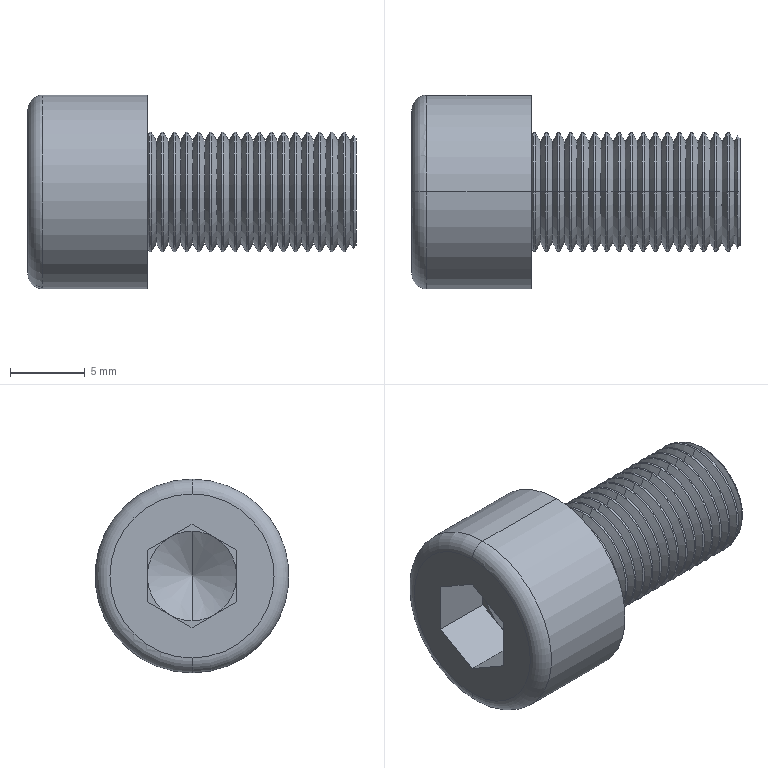Part | STEP file | PN_0011_Default<As Machined> | 1 solid | 148 faces | box 22 x 13 x 13 mm | volume 1485 mm3 | cone 84 | cylinder 42 | plane 20 | torus 2 | commonest cylinder face diameters 8 x34 9.353 x6 13 x2